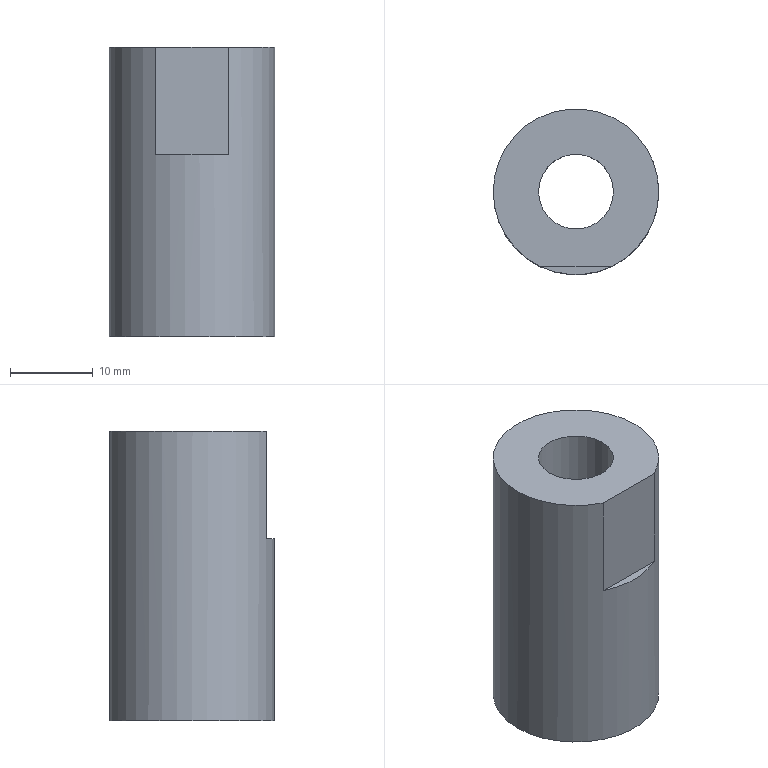Part | STEP file | lll_id314_x_t | 1 solid | 8 faces | box 20 x 20 x 35 mm | volume 7038 mm3 | plane 5 | cylinder 3 | commonest cylinder face diameters 9.05 x1 12.6 x1 20 x1
STEP:
#1=CARTESIAN_POINT('',(3686.141,-68.5,0.0000187));
#2=VERTEX_POINT('',#1);
#3=CARTESIAN_POINT('',(3694.859,-68.5,0.0000187));
#4=VERTEX_POINT('',#3);
#5=CARTESIAN_POINT('',(3690.5,-59.5,0.0000187));
#6=DIRECTION('',(0.,0.,-1.));
#7=DIRECTION('',(-1.,0.,0.));
#8=AXIS2_PLACEMENT_3D('',#5,#6,#7);
#9=CIRCLE('',#8,10.);
#10=EDGE_CURVE('',#2,#4,#9,.T.);
#11=ORIENTED_EDGE('',*,*,#10,.T.);
#12=CARTESIAN_POINT('',(3694.859,-68.5,-13.));
#13=VERTEX_POINT('',#12);
#14=CARTESIAN_POINT('',(3694.859,-68.5,-15.));
#15=DIRECTION('',(0.,0.,-1.));
#16=VECTOR('',#15,1.);
#17=LINE('',#14,#16);
#18=EDGE_CURVE('',#4,#13,#17,.T.);
#19=ORIENTED_EDGE('',*,*,#18,.T.);
#20=CARTESIAN_POINT('',(3686.141,-68.5,-13.));
#21=VERTEX_POINT('',#20);
#22=CARTESIAN_POINT('',(3690.5,-59.5,-13.));
#23=DIRECTION('',(0.,0.,1.));
#24=DIRECTION('',(-1.,0.,0.));
#25=AXIS2_PLACEMENT_3D('',#22,#23,#24);
#26=CIRCLE('',#25,10.);
#27=EDGE_CURVE('',#21,#13,#26,.T.);
#28=ORIENTED_EDGE('',*,*,#27,.F.);
#29=CARTESIAN_POINT('',(3686.141,-68.5,-15.));
#30=DIRECTION('',(0.,0.,1.));
#31=VECTOR('',#30,1.);
#32=LINE('',#29,#31);
#33=EDGE_CURVE('',#21,#2,#32,.T.);
#34=ORIENTED_EDGE('',*,*,#33,.T.);
#35=EDGE_LOOP('',(#11,#19,#28,#34));
#36=FACE_BOUND('',#35,.T.);
#37=CARTESIAN_POINT('',(3680.5,-59.5,-35.));
#38=VERTEX_POINT('',#37);
#39=CARTESIAN_POINT('',(3690.5,-59.5,-35.));
#40=DIRECTION('',(0.,0.,1.));
#41=DIRECTION('',(-1.,0.,0.));
#42=AXIS2_PLACEMENT_3D('',#39,#40,#41);
#43=CIRCLE('',#42,10.);
#44=EDGE_CURVE('',#38,#38,#43,.T.);
#45=ORIENTED_EDGE('',*,*,#44,.T.);
#46=EDGE_LOOP('',(#45));
#47=FACE_BOUND('',#46,.T.);
#48=CARTESIAN_POINT('',(3690.5,-59.5,-15.));
#49=DIRECTION('',(0.,0.,-1.));
#50=DIRECTION('',(0.,-1.,0.));
#51=AXIS2_PLACEMENT_3D('',#48,#49,#50);
#52=CYLINDRICAL_SURFACE('',#51,10.);
#53=ADVANCED_FACE('',(#36,#47),#52,.T.);
#54=CARTESIAN_POINT('',(3685.975,-59.5,0.0000187));
#55=VERTEX_POINT('',#54);
#56=CARTESIAN_POINT('',(3690.5,-59.5,0.0000187));
#57=DIRECTION('',(0.,0.,-1.));
#58=DIRECTION('',(-1.,0.,0.));
#59=AXIS2_PLACEMENT_3D('',#56,#57,#58);
#60=CIRCLE('',#59,4.525);
#61=EDGE_CURVE('',#55,#55,#60,.T.);
#62=ORIENTED_EDGE('',*,*,#61,.T.);
#63=EDGE_LOOP('',(#62));
#64=FACE_BOUND('',#63,.T.);
#65=ORIENTED_EDGE('',*,*,#10,.F.);
#66=CARTESIAN_POINT('',(3690.5,-68.5,0.0000187));
#67=DIRECTION('',(1.,0.,0.));
#68=VECTOR('',#67,1.);
#69=LINE('',#66,#68);
#70=EDGE_CURVE('',#2,#4,#69,.T.);
#71=ORIENTED_EDGE('',*,*,#70,.T.);
#72=EDGE_LOOP('',(#65,#71));
#73=FACE_BOUND('',#72,.T.);
#74=CARTESIAN_POINT('',(3690.5,-59.5,0.0000187));
#75=DIRECTION('',(0.,0.,1.));
#76=DIRECTION('',(1.,0.,0.));
#77=AXIS2_PLACEMENT_3D('',#74,#75,#76);
#78=PLANE('',#77);
#79=ADVANCED_FACE('',(#64,#73),#78,.T.);
#80=ORIENTED_EDGE('',*,*,#44,.F.);
#81=EDGE_LOOP('',(#80));
#82=FACE_BOUND('',#81,.T.);
#83=CARTESIAN_POINT('',(3696.8,-59.5,-35.));
#84=VERTEX_POINT('',#83);
#85=CARTESIAN_POINT('',(3690.5,-59.5,-35.));
#86=DIRECTION('',(0.,0.,-1.));
#87=DIRECTION('',(1.,0.,0.));
#88=AXIS2_PLACEMENT_3D('',#85,#86,#87);
#89=CIRCLE('',#88,6.3);
#90=EDGE_CURVE('',#84,#84,#89,.T.);
#91=ORIENTED_EDGE('',*,*,#90,.F.);
#92=EDGE_LOOP('',(#91));
#93=FACE_BOUND('',#92,.T.);
#94=CARTESIAN_POINT('',(3690.5,-65.,-35.));
#95=DIRECTION('',(0.,0.,-1.));
#96=DIRECTION('',(0.,1.,0.));
#97=AXIS2_PLACEMENT_3D('',#94,#95,#96);
#98=PLANE('',#97);
#99=ADVANCED_FACE('',(#82,#93),#98,.T.);
#100=CARTESIAN_POINT('',(3685.975,-59.5,-8.));
#101=VERTEX_POINT('',#100);
#102=CARTESIAN_POINT('',(3690.5,-59.5,-8.));
#103=DIRECTION('',(0.,0.,-1.));
#104=DIRECTION('',(-1.,0.,0.));
#105=AXIS2_PLACEMENT_3D('',#102,#103,#104);
#106=CIRCLE('',#105,4.525);
#107=EDGE_CURVE('',#101,#101,#106,.T.);
#108=ORIENTED_EDGE('',*,*,#107,.T.);
#109=EDGE_LOOP('',(#108));
#110=FACE_BOUND('',#109,.T.);
#111=ORIENTED_EDGE('',*,*,#61,.F.);
#112=EDGE_LOOP('',(#111));
#113=FACE_BOUND('',#112,.T.);
#114=CARTESIAN_POINT('',(3690.5,-59.5,-2.4));
#115=DIRECTION('',(0.,0.,1.));
#116=DIRECTION('',(-1.,0.,0.));
#117=AXIS2_PLACEMENT_3D('',#114,#115,#116);
#118=CYLINDRICAL_SURFACE('',#117,4.525);
#119=ADVANCED_FACE('',(#110,#113),#118,.F.);
#120=ORIENTED_EDGE('',*,*,#107,.F.);
#121=EDGE_LOOP('',(#120));
#122=FACE_BOUND('',#121,.T.);
#123=CARTESIAN_POINT('',(3684.2,-59.5,-8.));
#124=VERTEX_POINT('',#123);
#125=CARTESIAN_POINT('',(3690.5,-59.5,-8.));
#126=DIRECTION('',(0.,0.,1.));
#127=DIRECTION('',(-1.,0.,0.));
#128=AXIS2_PLACEMENT_3D('',#125,#126,#127);
#129=CIRCLE('',#128,6.3);
#130=EDGE_CURVE('',#124,#124,#129,.T.);
#131=ORIENTED_EDGE('',*,*,#130,.F.);
#132=EDGE_LOOP('',(#131));
#133=FACE_BOUND('',#132,.T.);
#134=CARTESIAN_POINT('',(3690.5,-59.5,-8.));
#135=DIRECTION('',(0.,0.,1.));
#136=DIRECTION('',(-1.,0.,0.));
#137=AXIS2_PLACEMENT_3D('',#134,#135,#136);
#138=PLANE('',#137);
#139=ADVANCED_FACE('',(#122,#133),#138,.F.);
#140=ORIENTED_EDGE('',*,*,#130,.T.);
#141=EDGE_LOOP('',(#140));
#142=FACE_BOUND('',#141,.T.);
#143=ORIENTED_EDGE('',*,*,#90,.T.);
#144=EDGE_LOOP('',(#143));
#145=FACE_BOUND('',#144,.T.);
#146=CARTESIAN_POINT('',(3690.5,-59.5,-35.));
#147=DIRECTION('',(0.,0.,1.));
#148=DIRECTION('',(-1.,0.,0.));
#149=AXIS2_PLACEMENT_3D('',#146,#147,#148);
#150=CYLINDRICAL_SURFACE('',#149,6.3);
#151=ADVANCED_FACE('',(#142,#145),#150,.F.);
#152=ORIENTED_EDGE('',*,*,#70,.F.);
#153=ORIENTED_EDGE('',*,*,#33,.F.);
#154=CARTESIAN_POINT('',(3682.5,-68.5,-13.));
#155=DIRECTION('',(1.,0.,0.));
#156=VECTOR('',#155,1.);
#157=LINE('',#154,#156);
#158=EDGE_CURVE('',#21,#13,#157,.T.);
#159=ORIENTED_EDGE('',*,*,#158,.T.);
#160=ORIENTED_EDGE('',*,*,#18,.F.);
#161=EDGE_LOOP('',(#152,#153,#159,#160));
#162=FACE_OUTER_BOUND('',#161,.T.);
#163=CARTESIAN_POINT('',(3690.5,-68.5,-1.));
#164=DIRECTION('',(0.,1.,0.));
#165=DIRECTION('',(0.,0.,1.));
#166=AXIS2_PLACEMENT_3D('',#163,#164,#165);
#167=PLANE('',#166);
#168=ADVANCED_FACE('',(#162),#167,.F.);
#169=ORIENTED_EDGE('',*,*,#27,.T.);
#170=ORIENTED_EDGE('',*,*,#158,.F.);
#171=EDGE_LOOP('',(#169,#170));
#172=FACE_OUTER_BOUND('',#171,.T.);
#173=CARTESIAN_POINT('',(3682.5,-76.5,-13.));
#174=DIRECTION('',(0.,0.,-1.));
#175=DIRECTION('',(-1.,0.,0.));
#176=AXIS2_PLACEMENT_3D('',#173,#174,#175);
#177=PLANE('',#176);
#178=ADVANCED_FACE('',(#172),#177,.F.);
#179=CLOSED_SHELL('',(#53,#79,#99,#119,#139,#151,#168,#178));
#180=MANIFOLD_SOLID_BREP('',#179);
#181=(LENGTH_UNIT()NAMED_UNIT(*)SI_UNIT(.MILLI.,.METRE.));
#182=UNCERTAINTY_MEASURE_WITH_UNIT(LENGTH_MEASURE(0.00002),#181,'','');
#183=(NAMED_UNIT(*)PLANE_ANGLE_UNIT()SI_UNIT($,.RADIAN.));
#184=PLANE_ANGLE_MEASURE_WITH_UNIT(PLANE_ANGLE_MEASURE(0.01745),#183);
#185=DIMENSIONAL_EXPONENTS(0.,0.,0.,0.,0.,0.,0.);
#186=(CONVERSION_BASED_UNIT('DEGREE',#184)NAMED_UNIT(#185)PLANE_ANGLE_UNIT());
#187=(NAMED_UNIT(*)SI_UNIT($,.STERADIAN.)SOLID_ANGLE_UNIT());
#188=(GEOMETRIC_REPRESENTATION_CONTEXT(3)GLOBAL_UNCERTAINTY_ASSIGNED_CONTEXT((#182))GLOBAL_UNIT_ASSIGNED_CONTEXT((#181,#186,#187))REPRESENTATION_CONTEXT('',''));
#189=ADVANCED_BREP_SHAPE_REPRESENTATION('',(#180),#188);